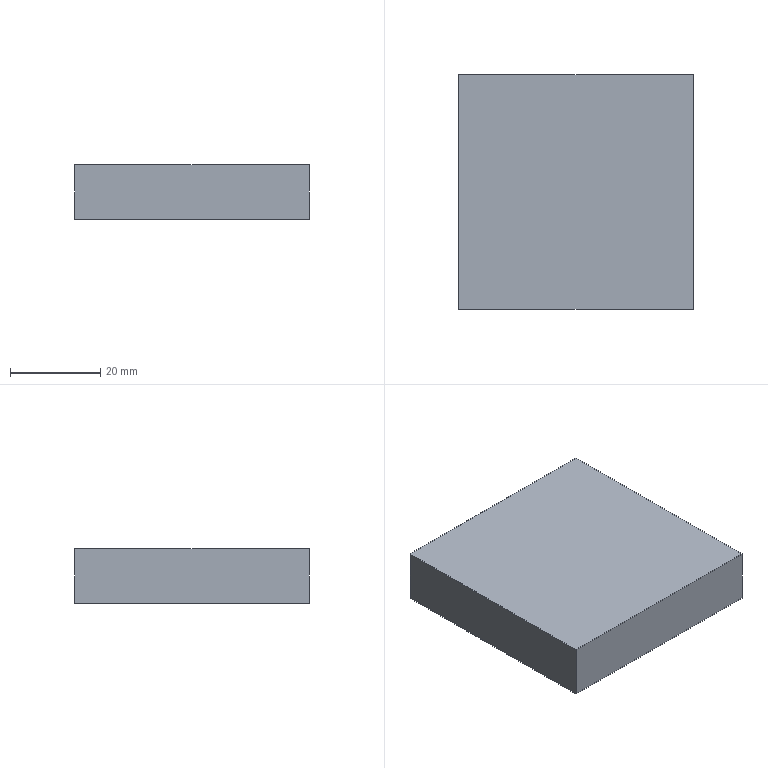Part | 2 solids | 127 faces | box 52 x 52 x 12 mm | volume 32340 mm3 | plane 44 | cone 42 | cylinder 25 | spline 16 | commonest cylinder face diameters 4 x8 5.3 x8 3.3 x4 42 x4 26.5 x1